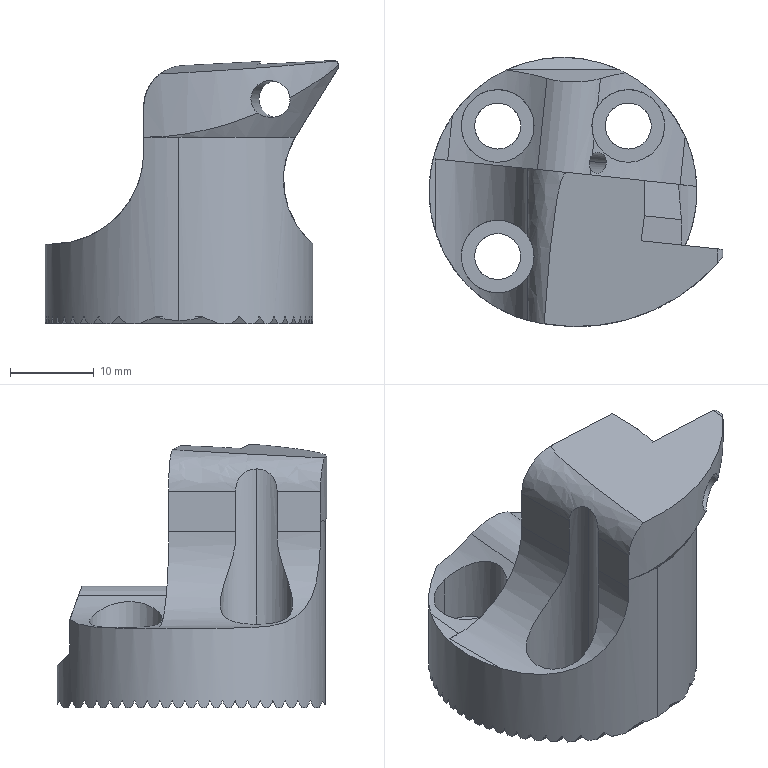NC program | Mastercam | posted with a generic post
Whole program:
%
:0001()
(MATERIAL - ALUMINUM MM - 2024)
(T10|50 FM |H10)
(T2|12 FEMR |H2|D2|WEAR COMP|TOOL DIA. - 12.|XY STOCK TO LEAVE - .5|Z STOCK TO LEAVE - 0.)
(T3|10 SPD |H3)
(T4|11 CBDR |H4)
(T11|5.5 CBDR |H11)
(T7|6 CBCHM |H7|D7|WEAR COMP|TOOL DIA. - 6.)
N100 G21
N102 G0 G17 G40 G80 G90 G94 G98
N104 G0 G28 G91 Z0.
N106 G0 G28 X0. Y0.
(50 FM |TOOL - 10|DIA. OFF. - 10|LEN. - 10|TOOL DIA. - 50.)
N108 T10 M6
N110 G0 G54 G90 X0. Y47.274 C0. B180. S1600 M3
N112 G43 H10 Z50.
N114 Z1.
N116 G1 Z0. F2000.
N118 Y19.774 F700.
N120 Y-19.774
N122 Y-47.274
N124 G0 Z50.
N126 M5
N128 G0 G28 G91 Z0.
N130 G28 B0.
N132 M01
N134 G0 G17 G40 G80 G90 G94 G98
N136 G0 G28 G91 Z0.
(12 FEMR |TOOL - 2|DIA. OFF. - 2|LEN. - 2|TOOL DIA. - 12.)
N138 T2 M6
N140 G0 G54 G90 X33.477 Y1.594 C0. B180. S3500 M3
N142 G43 H2 Z50.
N144 Z1.
N146 G1 Z-2. F2000.
N148 G41 D2 X23.479 Y1.416 F400.
N150 G3 X22.497 Y.417 I.017 J-.999
N152 X22.496 Y.399 I.999
N154 G2 X22.5 Y0. I-22.496 J-.399
N156 X0. Y-22.5 I-22.5
N158 X-22.5 Y0. J22.5
N160 X0. Y22.5 I22.5
N162 X22.496 Y.399 J-22.5
N164 X22.5 Y0. I-22.496 J-.399
N166 G1 X22.499 Y-.101
N168 X22.5 Y-.106
N170 G3 X23.495 Y-1.106 I1.
N172 G1 G40 X33.495 Y-1.151
N174 G0 Z50.
N176 M5
N178 G0 G28 G91 Z0.
N180 G28 B0.
N182 M01
N184 G0 G17 G40 G80 G90 G94 G98
N186 G0 G28 G91 Z0.
(10 SPD |TOOL - 3|DIA. OFF. - 3|LEN. - 3|TOOL DIA. - 10.)
N188 T3 M6
N190 G0 G54 G90 X7.8 Y-7.8 C0. B180. S2000 M3
N192 G43 H3 Z50.
N194 G81 G98 Z-3.5 R1. F100.
N196 Y7.8
N198 X-7.8
N200 G80
N202 M5
N204 G0 G28 G91 Z0.
N206 G28 B0.
N208 M01
N210 G0 G17 G40 G80 G90 G94 G98
N212 G0 G28 G91 Z0.
(11 CBDR |TOOL - 4|DIA. OFF. - 4|LEN. - 4|TOOL DIA. - 11.)
N214 T4 M6
N216 G0 G54 G90 X0. Y0. C0. B180. S2000 M3
N218 G43 H4 Z50.
N220 G81 G98 Z-8. R1. F100.
N222 G80
N224 M5
N226 G0 G28 G91 Z0.
N228 G28 B0.
N230 M01
N232 G0 G17 G40 G80 G90 G94 G98
N234 G0 G28 G91 Z0.
(5.5 CBDR |TOOL - 11|DIA. OFF. - 11|LEN. - 11|TOOL DIA. - 5.5)
N236 T11 M6
N238 G0 G54 G90 X7.8 Y-7.8 C0. B180. S2200 M3
N240 G43 H11 Z50.
N242 G81 G98 Z-15. R1. F60.
N244 Y7.8
N246 X-7.8
N248 G80
N250 M5
N252 G0 G28 G91 Z0.
N254 G28 B0.
N256 M01
N258 G0 G17 G40 G80 G90 G94 G98
N260 G0 G28 G91 Z0.
(6 CBCHM |TOOL - 7|DIA. OFF. - 7|LEN. - 7|TOOL DIA. - 6.)
N262 T7 M6
N264 G0 G54 G90 X22.187 Y.9 C0. B180. S3500 M3
N266 G43 H7 Z50.
N268 Z1.
N270 G1 Z-1.7 F2000.
N272 G41 D7 X17.188 Y.81 F400.
N274 G3 X16.697 Y.31 I.009 J-.5
N276 G1 Y.301
N278 G2 X16.7 Y0. I-16.697 J-.301
N280 X0. Y-16.7 I-16.7
N282 X-16.7 Y0. J16.7
N284 X0. Y16.7 I16.7
N286 X16.697 Y.301 J-16.7
N288 X16.7 Y0. I-16.697 J-.301
N290 X16.699 Y-.199 I-16.7
N292 G1 Y-.205
N294 G3 X17.193 Y-.705 I.5
N296 G1 G40 X22.192 Y-.764
N298 G0 Z50.
N300 X-1.5 Y.5
N302 Z1.
N304 G1 Z-2. F2000.
N306 G41 D7 X-4.5 F400.
N308 G3 X-5. Y0. J-.5
N310 X0. Y-5. I5.
N312 X5. Y0. J5.
N314 X0. Y5. I-5.
N316 X-5. Y0. J-5.
N318 X-4.975 Y-.499 I5.
N320 X-4.478 Y-.949 I.497 J.05
N322 X-4.428 Y-.947 J.5
N324 G1 G40 X-1.443 Y-.647
N326 G0 Z50.
N328 M5
N330 G0 G28 G91 Z0.
N332 G0 G28 X0. Y0.
N334 G28 B0.
N336 M30
%